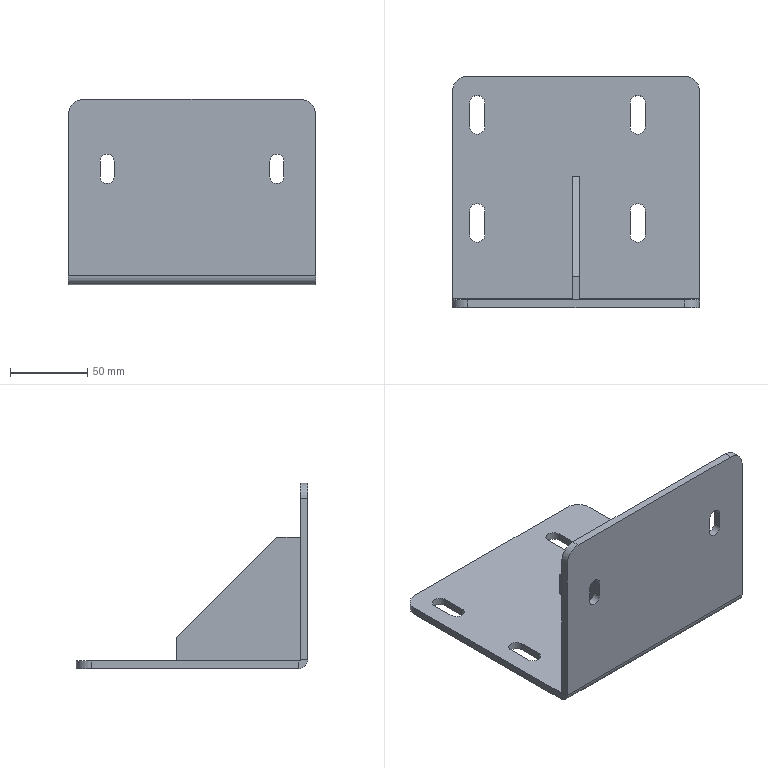Part | SolidWorks | features ICE 3, EdgeFlange 1, Fillet 1, FlatPattern 1, Gusset 1, SMBaseFlange 1, SheetMetal 1 | 2 solids | 51 faces | box 160 x 150 x 120 mm | volume 225790 mm3 | plane 31 | cylinder 20 | commonest cylinder face diameters 10 x8 9 x6 20 x4 1.473 x1 11.473 x1
STEP:
#1=CARTESIAN_POINT('',(-2.5,80.,-55.));
#2=VERTEX_POINT('',#1);
#3=CARTESIAN_POINT('',(-2.5,80.,-40.));
#4=VERTEX_POINT('',#3);
#5=CARTESIAN_POINT('',(-2.5,80.,-55.));
#6=DIRECTION('',(0.,0.,1.));
#7=VECTOR('',#6,1000.);
#8=LINE('',#5,#7);
#9=EDGE_CURVE('',#2,#4,#8,.T.);
#10=ORIENTED_EDGE('',*,*,#9,.T.);
#11=CARTESIAN_POINT('',(2.5,80.,-40.));
#12=VERTEX_POINT('',#11);
#13=CARTESIAN_POINT('',(2.5,80.,-40.));
#14=DIRECTION('',(-1.,0.,0.));
#15=VECTOR('',#14,1000.);
#16=LINE('',#13,#15);
#17=EDGE_CURVE('',#12,#4,#16,.T.);
#18=ORIENTED_EDGE('',*,*,#17,.F.);
#19=CARTESIAN_POINT('',(2.5,80.,-55.));
#20=VERTEX_POINT('',#19);
#21=CARTESIAN_POINT('',(2.5,80.,-55.));
#22=DIRECTION('',(0.,0.,1.));
#23=VECTOR('',#22,1000.);
#24=LINE('',#21,#23);
#25=EDGE_CURVE('',#20,#12,#24,.T.);
#26=ORIENTED_EDGE('',*,*,#25,.F.);
#27=CARTESIAN_POINT('',(2.5,80.,-55.));
#28=DIRECTION('',(-1.,0.,0.));
#29=VECTOR('',#28,1000.);
#30=LINE('',#27,#29);
#31=EDGE_CURVE('',#20,#2,#30,.T.);
#32=ORIENTED_EDGE('',*,*,#31,.T.);
#33=EDGE_LOOP('',(#10,#18,#26,#32));
#34=FACE_OUTER_BOUND('',#33,.T.);
#35=CARTESIAN_POINT('',(2.5,80.,-55.));
#36=DIRECTION('',(0.,-1.,0.));
#37=DIRECTION('',(0.,0.,-1.));
#38=AXIS2_PLACEMENT_3D('',#35,#36,#37);
#39=PLANE('',#38);
#40=ADVANCED_FACE('',(#34),#39,.F.);
#41=CARTESIAN_POINT('',(-2.5,15.,25.));
#42=VERTEX_POINT('',#41);
#43=CARTESIAN_POINT('',(-2.5,80.,-40.));
#44=DIRECTION('',(0.,-0.7071,0.7071));
#45=VECTOR('',#44,1000.);
#46=LINE('',#43,#45);
#47=EDGE_CURVE('',#4,#42,#46,.T.);
#48=ORIENTED_EDGE('',*,*,#47,.T.);
#49=CARTESIAN_POINT('',(2.5,15.,25.));
#50=VERTEX_POINT('',#49);
#51=CARTESIAN_POINT('',(2.5,15.,25.));
#52=DIRECTION('',(-1.,0.,0.));
#53=VECTOR('',#52,1000.);
#54=LINE('',#51,#53);
#55=EDGE_CURVE('',#50,#42,#54,.T.);
#56=ORIENTED_EDGE('',*,*,#55,.F.);
#57=CARTESIAN_POINT('',(2.5,80.,-40.));
#58=DIRECTION('',(0.,-0.7071,0.7071));
#59=VECTOR('',#58,1000.);
#60=LINE('',#57,#59);
#61=EDGE_CURVE('',#12,#50,#60,.T.);
#62=ORIENTED_EDGE('',*,*,#61,.F.);
#63=ORIENTED_EDGE('',*,*,#17,.T.);
#64=EDGE_LOOP('',(#48,#56,#62,#63));
#65=FACE_OUTER_BOUND('',#64,.T.);
#66=CARTESIAN_POINT('',(2.5,80.,-40.));
#67=DIRECTION('',(0.,-0.7071,-0.7071));
#68=DIRECTION('',(0.,0.7071,-0.7071));
#69=AXIS2_PLACEMENT_3D('',#66,#67,#68);
#70=PLANE('',#69);
#71=ADVANCED_FACE('',(#65),#70,.F.);
#72=CARTESIAN_POINT('',(-2.5,0.,25.));
#73=VERTEX_POINT('',#72);
#74=CARTESIAN_POINT('',(-2.5,0.,25.));
#75=DIRECTION('',(0.,-1.,0.));
#76=VECTOR('',#75,1000.);
#77=LINE('',#74,#76);
#78=EDGE_CURVE('',#42,#73,#77,.T.);
#79=ORIENTED_EDGE('',*,*,#78,.T.);
#80=CARTESIAN_POINT('',(2.5,0.,25.));
#81=VERTEX_POINT('',#80);
#82=CARTESIAN_POINT('',(2.5,0.,25.));
#83=DIRECTION('',(-1.,0.,0.));
#84=VECTOR('',#83,1000.);
#85=LINE('',#82,#84);
#86=EDGE_CURVE('',#81,#73,#85,.T.);
#87=ORIENTED_EDGE('',*,*,#86,.F.);
#88=CARTESIAN_POINT('',(2.5,0.,25.));
#89=DIRECTION('',(0.,-1.,0.));
#90=VECTOR('',#89,1000.);
#91=LINE('',#88,#90);
#92=EDGE_CURVE('',#50,#81,#91,.T.);
#93=ORIENTED_EDGE('',*,*,#92,.F.);
#94=ORIENTED_EDGE('',*,*,#55,.T.);
#95=EDGE_LOOP('',(#79,#87,#93,#94));
#96=FACE_OUTER_BOUND('',#95,.T.);
#97=CARTESIAN_POINT('',(2.5,0.,25.));
#98=DIRECTION('',(0.,0.,-1.));
#99=DIRECTION('',(-1.,0.,0.));
#100=AXIS2_PLACEMENT_3D('',#97,#98,#99);
#101=PLANE('',#100);
#102=ADVANCED_FACE('',(#96),#101,.F.);
#103=CARTESIAN_POINT('',(-2.5,0.,-55.));
#104=VERTEX_POINT('',#103);
#105=CARTESIAN_POINT('',(-2.5,0.,-55.));
#106=DIRECTION('',(0.,0.,-1.));
#107=VECTOR('',#106,1000.);
#108=LINE('',#105,#107);
#109=EDGE_CURVE('',#73,#104,#108,.T.);
#110=ORIENTED_EDGE('',*,*,#109,.T.);
#111=CARTESIAN_POINT('',(2.5,0.,-55.));
#112=VERTEX_POINT('',#111);
#113=CARTESIAN_POINT('',(2.5,0.,-55.));
#114=DIRECTION('',(-1.,0.,0.));
#115=VECTOR('',#114,1000.);
#116=LINE('',#113,#115);
#117=EDGE_CURVE('',#112,#104,#116,.T.);
#118=ORIENTED_EDGE('',*,*,#117,.F.);
#119=CARTESIAN_POINT('',(2.5,0.,-55.));
#120=DIRECTION('',(0.,0.,-1.));
#121=VECTOR('',#120,1000.);
#122=LINE('',#119,#121);
#123=EDGE_CURVE('',#81,#112,#122,.T.);
#124=ORIENTED_EDGE('',*,*,#123,.F.);
#125=ORIENTED_EDGE('',*,*,#86,.T.);
#126=EDGE_LOOP('',(#110,#118,#124,#125));
#127=FACE_OUTER_BOUND('',#126,.T.);
#128=CARTESIAN_POINT('',(2.5,0.,-55.));
#129=DIRECTION('',(0.,1.,0.));
#130=DIRECTION('',(0.,0.,1.));
#131=AXIS2_PLACEMENT_3D('',#128,#129,#130);
#132=PLANE('',#131);
#133=ADVANCED_FACE('',(#127),#132,.F.);
#134=CARTESIAN_POINT('',(-2.5,0.,-55.));
#135=DIRECTION('',(0.,1.,0.));
#136=VECTOR('',#135,1000.);
#137=LINE('',#134,#136);
#138=EDGE_CURVE('',#104,#2,#137,.T.);
#139=ORIENTED_EDGE('',*,*,#138,.T.);
#140=ORIENTED_EDGE('',*,*,#31,.F.);
#141=CARTESIAN_POINT('',(2.5,0.,-55.));
#142=DIRECTION('',(0.,1.,0.));
#143=VECTOR('',#142,1000.);
#144=LINE('',#141,#143);
#145=EDGE_CURVE('',#112,#20,#144,.T.);
#146=ORIENTED_EDGE('',*,*,#145,.F.);
#147=ORIENTED_EDGE('',*,*,#117,.T.);
#148=EDGE_LOOP('',(#139,#140,#146,#147));
#149=FACE_OUTER_BOUND('',#148,.T.);
#150=CARTESIAN_POINT('',(2.5,0.,-55.));
#151=DIRECTION('',(0.,0.,1.));
#152=DIRECTION('',(1.,0.,0.));
#153=AXIS2_PLACEMENT_3D('',#150,#151,#152);
#154=PLANE('',#153);
#155=ADVANCED_FACE('',(#149),#154,.F.);
#156=ORIENTED_EDGE('',*,*,#25,.T.);
#157=ORIENTED_EDGE('',*,*,#61,.T.);
#158=ORIENTED_EDGE('',*,*,#92,.T.);
#159=ORIENTED_EDGE('',*,*,#123,.T.);
#160=ORIENTED_EDGE('',*,*,#145,.T.);
#161=EDGE_LOOP('',(#156,#157,#158,#159,#160));
#162=FACE_OUTER_BOUND('',#161,.T.);
#163=CARTESIAN_POINT('',(2.5,0.,0.));
#164=DIRECTION('',(-1.,0.,0.));
#165=DIRECTION('',(0.,0.,1.));
#166=AXIS2_PLACEMENT_3D('',#163,#164,#165);
#167=PLANE('',#166);
#168=ADVANCED_FACE('',(#162),#167,.F.);
#169=ORIENTED_EDGE('',*,*,#9,.F.);
#170=ORIENTED_EDGE('',*,*,#138,.F.);
#171=ORIENTED_EDGE('',*,*,#109,.F.);
#172=ORIENTED_EDGE('',*,*,#78,.F.);
#173=ORIENTED_EDGE('',*,*,#47,.F.);
#174=EDGE_LOOP('',(#169,#170,#171,#172,#173));
#175=FACE_OUTER_BOUND('',#174,.T.);
#176=CARTESIAN_POINT('',(-2.5,0.,0.));
#177=DIRECTION('',(-1.,0.,0.));
#178=DIRECTION('',(0.,0.,1.));
#179=AXIS2_PLACEMENT_3D('',#176,#177,#178);
#180=PLANE('',#179);
#181=ADVANCED_FACE('',(#175),#180,.T.);
#182=CLOSED_SHELL('',(#40,#71,#102,#133,#155,#168,#181));
#183=MANIFOLD_SOLID_BREP('',#182);
#184=CARTESIAN_POINT('',(-55.,-5.,24.5));
#185=VERTEX_POINT('',#184);
#186=CARTESIAN_POINT('',(-50.5,-5.,20.));
#187=VERTEX_POINT('',#186);
#188=CARTESIAN_POINT('',(-55.,-5.,20.));
#189=DIRECTION('',(0.,1.,0.));
#190=DIRECTION('',(0.,0.,1.));
#191=AXIS2_PLACEMENT_3D('',#188,#189,#190);
#192=CIRCLE('',#191,4.5);
#193=EDGE_CURVE('',#185,#187,#192,.T.);
#194=ORIENTED_EDGE('',*,*,#193,.F.);
#195=CARTESIAN_POINT('',(-55.,0.,24.5));
#196=VERTEX_POINT('',#195);
#197=CARTESIAN_POINT('',(-55.,-5.,24.5));
#198=DIRECTION('',(0.,1.,0.));
#199=VECTOR('',#198,1000.);
#200=LINE('',#197,#199);
#201=EDGE_CURVE('',#185,#196,#200,.T.);
#202=ORIENTED_EDGE('',*,*,#201,.T.);
#203=CARTESIAN_POINT('',(-50.5,0.,20.));
#204=VERTEX_POINT('',#203);
#205=CARTESIAN_POINT('',(-55.,0.,20.));
#206=DIRECTION('',(0.,1.,0.));
#207=DIRECTION('',(0.,0.,1.));
#208=AXIS2_PLACEMENT_3D('',#205,#206,#207);
#209=CIRCLE('',#208,4.5);
#210=EDGE_CURVE('',#196,#204,#209,.T.);
#211=ORIENTED_EDGE('',*,*,#210,.T.);
#212=CARTESIAN_POINT('',(-50.5,-5.,20.));
#213=DIRECTION('',(0.,1.,0.));
#214=VECTOR('',#213,1000.);
#215=LINE('',#212,#214);
#216=EDGE_CURVE('',#187,#204,#215,.T.);
#217=ORIENTED_EDGE('',*,*,#216,.F.);
#218=EDGE_LOOP('',(#194,#202,#211,#217));
#219=FACE_OUTER_BOUND('',#218,.T.);
#220=CARTESIAN_POINT('',(-55.,-5.,20.));
#221=DIRECTION('',(0.,1.,0.));
#222=DIRECTION('',(0.,0.,1.));
#223=AXIS2_PLACEMENT_3D('',#220,#221,#222);
#224=CYLINDRICAL_SURFACE('',#223,4.5);
#225=ADVANCED_FACE('',(#219),#224,.F.);
#226=CARTESIAN_POINT('',(55.,-5.,24.5));
#227=VERTEX_POINT('',#226);
#228=CARTESIAN_POINT('',(59.5,-5.,20.));
#229=VERTEX_POINT('',#228);
#230=CARTESIAN_POINT('',(55.,-5.,20.));
#231=DIRECTION('',(0.,1.,0.));
#232=DIRECTION('',(0.,0.,1.));
#233=AXIS2_PLACEMENT_3D('',#230,#231,#232);
#234=CIRCLE('',#233,4.5);
#235=EDGE_CURVE('',#227,#229,#234,.T.);
#236=ORIENTED_EDGE('',*,*,#235,.F.);
#237=CARTESIAN_POINT('',(55.,0.,24.5));
#238=VERTEX_POINT('',#237);
#239=CARTESIAN_POINT('',(55.,-5.,24.5));
#240=DIRECTION('',(0.,1.,0.));
#241=VECTOR('',#240,1000.);
#242=LINE('',#239,#241);
#243=EDGE_CURVE('',#227,#238,#242,.T.);
#244=ORIENTED_EDGE('',*,*,#243,.T.);
#245=CARTESIAN_POINT('',(59.5,0.,20.));
#246=VERTEX_POINT('',#245);
#247=CARTESIAN_POINT('',(55.,0.,20.));
#248=DIRECTION('',(0.,1.,0.));
#249=DIRECTION('',(0.,0.,1.));
#250=AXIS2_PLACEMENT_3D('',#247,#248,#249);
#251=CIRCLE('',#250,4.5);
#252=EDGE_CURVE('',#238,#246,#251,.T.);
#253=ORIENTED_EDGE('',*,*,#252,.T.);
#254=CARTESIAN_POINT('',(59.5,-5.,20.));
#255=DIRECTION('',(0.,1.,0.));
#256=VECTOR('',#255,1000.);
#257=LINE('',#254,#256);
#258=EDGE_CURVE('',#229,#246,#257,.T.);
#259=ORIENTED_EDGE('',*,*,#258,.F.);
#260=EDGE_LOOP('',(#236,#244,#253,#259));
#261=FACE_OUTER_BOUND('',#260,.T.);
#262=CARTESIAN_POINT('',(55.,-5.,20.));
#263=DIRECTION('',(0.,1.,0.));
#264=DIRECTION('',(0.,0.,1.));
#265=AXIS2_PLACEMENT_3D('',#262,#263,#264);
#266=CYLINDRICAL_SURFACE('',#265,4.5);
#267=ADVANCED_FACE('',(#261),#266,.F.);
#268=CARTESIAN_POINT('',(-80.,0.,-54.263));
#269=VERTEX_POINT('',#268);
#270=CARTESIAN_POINT('',(-80.,0.,50.));
#271=VERTEX_POINT('',#270);
#272=CARTESIAN_POINT('',(-80.,0.,50.));
#273=DIRECTION('',(0.,0.,1.));
#274=VECTOR('',#273,1000.);
#275=LINE('',#272,#274);
#276=EDGE_CURVE('',#269,#271,#275,.T.);
#277=ORIENTED_EDGE('',*,*,#276,.F.);
#278=CARTESIAN_POINT('',(-80.,-5.,-54.263));
#279=VERTEX_POINT('',#278);
#280=CARTESIAN_POINT('',(-80.,0.,-54.263));
#281=DIRECTION('',(0.,-1.,0.));
#282=VECTOR('',#281,1000.);
#283=LINE('',#280,#282);
#284=EDGE_CURVE('',#269,#279,#283,.T.);
#285=ORIENTED_EDGE('',*,*,#284,.T.);
#286=CARTESIAN_POINT('',(-80.,-5.,50.));
#287=VERTEX_POINT('',#286);
#288=CARTESIAN_POINT('',(-80.,-5.,50.));
#289=DIRECTION('',(0.,0.,1.));
#290=VECTOR('',#289,1000.);
#291=LINE('',#288,#290);
#292=EDGE_CURVE('',#279,#287,#291,.T.);
#293=ORIENTED_EDGE('',*,*,#292,.T.);
#294=CARTESIAN_POINT('',(-80.,-5.,50.));
#295=DIRECTION('',(0.,1.,0.));
#296=VECTOR('',#295,1000.);
#297=LINE('',#294,#296);
#298=EDGE_CURVE('',#287,#271,#297,.T.);
#299=ORIENTED_EDGE('',*,*,#298,.T.);
#300=EDGE_LOOP('',(#277,#285,#293,#299));
#301=FACE_OUTER_BOUND('',#300,.T.);
#302=CARTESIAN_POINT('',(-80.,-5.,50.));
#303=DIRECTION('',(-1.,0.,0.));
#304=DIRECTION('',(0.,0.,1.));
#305=AXIS2_PLACEMENT_3D('',#302,#303,#304);
#306=PLANE('',#305);
#307=ADVANCED_FACE('',(#301),#306,.T.);
#308=CARTESIAN_POINT('',(-50.5,-5.,10.));
#309=VERTEX_POINT('',#308);
#310=CARTESIAN_POINT('',(-59.5,-5.,10.));
#311=VERTEX_POINT('',#310);
#312=CARTESIAN_POINT('',(-55.,-5.,10.));
#313=DIRECTION('',(0.,1.,0.));
#314=DIRECTION('',(0.,0.,1.));
#315=AXIS2_PLACEMENT_3D('',#312,#313,#314);
#316=CIRCLE('',#315,4.5);
#317=EDGE_CURVE('',#309,#311,#316,.T.);
#318=ORIENTED_EDGE('',*,*,#317,.T.);
#319=CARTESIAN_POINT('',(-59.5,-5.,20.));
#320=VERTEX_POINT('',#319);
#321=CARTESIAN_POINT('',(-59.5,-5.,10.));
#322=DIRECTION('',(0.,0.,1.));
#323=VECTOR('',#322,1000.);
#324=LINE('',#321,#323);
#325=EDGE_CURVE('',#311,#320,#324,.T.);
#326=ORIENTED_EDGE('',*,*,#325,.T.);
#327=CARTESIAN_POINT('',(-55.,-5.,20.));
#328=DIRECTION('',(0.,1.,0.));
#329=DIRECTION('',(0.,0.,1.));
#330=AXIS2_PLACEMENT_3D('',#327,#328,#329);
#331=CIRCLE('',#330,4.5);
#332=EDGE_CURVE('',#320,#185,#331,.T.);
#333=ORIENTED_EDGE('',*,*,#332,.T.);
#334=ORIENTED_EDGE('',*,*,#193,.T.);
#335=CARTESIAN_POINT('',(-50.5,-5.,10.));
#336=DIRECTION('',(0.,0.,-1.));
#337=VECTOR('',#336,1000.);
#338=LINE('',#335,#337);
#339=EDGE_CURVE('',#187,#309,#338,.T.);
#340=ORIENTED_EDGE('',*,*,#339,.T.);
#341=EDGE_LOOP('',(#318,#326,#333,#334,#340));
#342=FACE_BOUND('',#341,.T.);
#343=CARTESIAN_POINT('',(59.5,-5.,10.));
#344=VERTEX_POINT('',#343);
#345=CARTESIAN_POINT('',(50.5,-5.,10.));
#346=VERTEX_POINT('',#345);
#347=CARTESIAN_POINT('',(55.,-5.,10.));
#348=DIRECTION('',(0.,1.,0.));
#349=DIRECTION('',(0.,0.,1.));
#350=AXIS2_PLACEMENT_3D('',#347,#348,#349);
#351=CIRCLE('',#350,4.5);
#352=EDGE_CURVE('',#344,#346,#351,.T.);
#353=ORIENTED_EDGE('',*,*,#352,.T.);
#354=CARTESIAN_POINT('',(50.5,-5.,20.));
#355=VERTEX_POINT('',#354);
#356=CARTESIAN_POINT('',(50.5,-5.,10.));
#357=DIRECTION('',(0.,0.,1.));
#358=VECTOR('',#357,1000.);
#359=LINE('',#356,#358);
#360=EDGE_CURVE('',#346,#355,#359,.T.);
#361=ORIENTED_EDGE('',*,*,#360,.T.);
#362=CARTESIAN_POINT('',(55.,-5.,20.));
#363=DIRECTION('',(0.,1.,0.));
#364=DIRECTION('',(0.,0.,1.));
#365=AXIS2_PLACEMENT_3D('',#362,#363,#364);
#366=CIRCLE('',#365,4.5);
#367=EDGE_CURVE('',#355,#227,#366,.T.);
#368=ORIENTED_EDGE('',*,*,#367,.T.);
#369=ORIENTED_EDGE('',*,*,#235,.T.);
#370=CARTESIAN_POINT('',(59.5,-5.,10.));
#371=DIRECTION('',(0.,0.,-1.));
#372=VECTOR('',#371,1000.);
#373=LINE('',#370,#372);
#374=EDGE_CURVE('',#229,#344,#373,.T.);
#375=ORIENTED_EDGE('',*,*,#374,.T.);
#376=EDGE_LOOP('',(#353,#361,#368,#369,#375));
#377=FACE_BOUND('',#376,.T.);
#378=ORIENTED_EDGE('',*,*,#292,.F.);
#379=CARTESIAN_POINT('',(80.,-5.,-54.263));
#380=VERTEX_POINT('',#379);
#381=CARTESIAN_POINT('',(-80.,-5.,-54.263));
#382=DIRECTION('',(1.,0.,0.));
#383=VECTOR('',#382,1000.);
#384=LINE('',#381,#383);
#385=EDGE_CURVE('',#279,#380,#384,.T.);
#386=ORIENTED_EDGE('',*,*,#385,.T.);
#387=CARTESIAN_POINT('',(80.,-5.,50.));
#388=VERTEX_POINT('',#387);
#389=CARTESIAN_POINT('',(80.,-5.,50.));
#390=DIRECTION('',(0.,0.,-1.));
#391=VECTOR('',#390,1000.);
#392=LINE('',#389,#391);
#393=EDGE_CURVE('',#388,#380,#392,.T.);
#394=ORIENTED_EDGE('',*,*,#393,.F.);
#395=CARTESIAN_POINT('',(70.,-5.,60.));
#396=VERTEX_POINT('',#395);
#397=CARTESIAN_POINT('',(70.,-5.,50.));
#398=DIRECTION('',(0.,1.,0.));
#399=DIRECTION('',(0.,0.,-1.));
#400=AXIS2_PLACEMENT_3D('',#397,#398,#399);
#401=CIRCLE('',#400,10.);
#402=EDGE_CURVE('',#396,#388,#401,.T.);
#403=ORIENTED_EDGE('',*,*,#402,.F.);
#404=CARTESIAN_POINT('',(-70.,-5.,60.));
#405=VERTEX_POINT('',#404);
#406=CARTESIAN_POINT('',(-70.,-5.,60.));
#407=DIRECTION('',(1.,0.,0.));
#408=VECTOR('',#407,1000.);
#409=LINE('',#406,#408);
#410=EDGE_CURVE('',#405,#396,#409,.T.);
#411=ORIENTED_EDGE('',*,*,#410,.F.);
#412=CARTESIAN_POINT('',(-70.,-5.,50.));
#413=DIRECTION('',(0.,1.,0.));
#414=DIRECTION('',(0.,0.,-1.));
#415=AXIS2_PLACEMENT_3D('',#412,#413,#414);
#416=CIRCLE('',#415,10.);
#417=EDGE_CURVE('',#287,#405,#416,.T.);
#418=ORIENTED_EDGE('',*,*,#417,.F.);
#419=EDGE_LOOP('',(#378,#386,#394,#403,#411,#418));
#420=FACE_OUTER_BOUND('',#419,.T.);
#421=CARTESIAN_POINT('',(-70.,-5.,50.));
#422=DIRECTION('',(0.,-1.,0.));
#423=DIRECTION('',(0.,0.,-1.));
#424=AXIS2_PLACEMENT_3D('',#421,#422,#423);
#425=PLANE('',#424);
#426=ADVANCED_FACE('',(#342,#377,#420),#425,.T.);
#427=CARTESIAN_POINT('',(-59.5,0.,10.));
#428=VERTEX_POINT('',#427);
#429=CARTESIAN_POINT('',(-59.5,0.,20.));
#430=VERTEX_POINT('',#429);
#431=CARTESIAN_POINT('',(-59.5,0.,10.));
#432=DIRECTION('',(0.,0.,1.));
#433=VECTOR('',#432,1000.);
#434=LINE('',#431,#433);
#435=EDGE_CURVE('',#428,#430,#434,.T.);
#436=ORIENTED_EDGE('',*,*,#435,.F.);
#437=CARTESIAN_POINT('',(-50.5,0.,10.));
#438=VERTEX_POINT('',#437);
#439=CARTESIAN_POINT('',(-55.,0.,10.));
#440=DIRECTION('',(0.,1.,0.));
#441=DIRECTION('',(0.,0.,1.));
#442=AXIS2_PLACEMENT_3D('',#439,#440,#441);
#443=CIRCLE('',#442,4.5);
#444=EDGE_CURVE('',#438,#428,#443,.T.);
#445=ORIENTED_EDGE('',*,*,#444,.F.);
#446=CARTESIAN_POINT('',(-50.5,0.,10.));
#447=DIRECTION('',(0.,0.,-1.));
#448=VECTOR('',#447,1000.);
#449=LINE('',#446,#448);
#450=EDGE_CURVE('',#204,#438,#449,.T.);
#451=ORIENTED_EDGE('',*,*,#450,.F.);
#452=ORIENTED_EDGE('',*,*,#210,.F.);
#453=CARTESIAN_POINT('',(-55.,0.,20.));
#454=DIRECTION('',(0.,1.,0.));
#455=DIRECTION('',(0.,0.,1.));
#456=AXIS2_PLACEMENT_3D('',#453,#454,#455);
#457=CIRCLE('',#456,4.5);
#458=EDGE_CURVE('',#430,#196,#457,.T.);
#459=ORIENTED_EDGE('',*,*,#458,.F.);
#460=EDGE_LOOP('',(#436,#445,#451,#452,#459));
#461=FACE_BOUND('',#460,.T.);
#462=CARTESIAN_POINT('',(50.5,0.,10.));
#463=VERTEX_POINT('',#462);
#464=CARTESIAN_POINT('',(50.5,0.,20.));
#465=VERTEX_POINT('',#464);
#466=CARTESIAN_POINT('',(50.5,0.,10.));
#467=DIRECTION('',(0.,0.,1.));
#468=VECTOR('',#467,1000.);
#469=LINE('',#466,#468);
#470=EDGE_CURVE('',#463,#465,#469,.T.);
#471=ORIENTED_EDGE('',*,*,#470,.F.);
#472=CARTESIAN_POINT('',(59.5,0.,10.));
#473=VERTEX_POINT('',#472);
#474=CARTESIAN_POINT('',(55.,0.,10.));
#475=DIRECTION('',(0.,1.,0.));
#476=DIRECTION('',(0.,0.,1.));
#477=AXIS2_PLACEMENT_3D('',#474,#475,#476);
#478=CIRCLE('',#477,4.5);
#479=EDGE_CURVE('',#473,#463,#478,.T.);
#480=ORIENTED_EDGE('',*,*,#479,.F.);
#481=CARTESIAN_POINT('',(59.5,0.,10.));
#482=DIRECTION('',(0.,0.,-1.));
#483=VECTOR('',#482,1000.);
#484=LINE('',#481,#483);
#485=EDGE_CURVE('',#246,#473,#484,.T.);
#486=ORIENTED_EDGE('',*,*,#485,.F.);
#487=ORIENTED_EDGE('',*,*,#252,.F.);
#488=CARTESIAN_POINT('',(55.,0.,20.));
#489=DIRECTION('',(0.,1.,0.));
#490=DIRECTION('',(0.,0.,1.));
#491=AXIS2_PLACEMENT_3D('',#488,#489,#490);
#492=CIRCLE('',#491,4.5);
#493=EDGE_CURVE('',#465,#238,#492,.T.);
#494=ORIENTED_EDGE('',*,*,#493,.F.);
#495=EDGE_LOOP('',(#471,#480,#486,#487,#494));
#496=FACE_BOUND('',#495,.T.);
#497=CARTESIAN_POINT('',(80.,0.,-54.263));
#498=VERTEX_POINT('',#497);
#499=CARTESIAN_POINT('',(-80.,0.,-54.263));
#500=DIRECTION('',(1.,0.,0.));
#501=VECTOR('',#500,1000.);
#502=LINE('',#499,#501);
#503=EDGE_CURVE('',#269,#498,#502,.T.);
#504=ORIENTED_EDGE('',*,*,#503,.F.);
#505=ORIENTED_EDGE('',*,*,#276,.T.);
#506=CARTESIAN_POINT('',(-70.,0.,60.));
#507=VERTEX_POINT('',#506);
#508=CARTESIAN_POINT('',(-70.,0.,50.));
#509=DIRECTION('',(0.,1.,0.));
#510=DIRECTION('',(0.,0.,-1.));
#511=AXIS2_PLACEMENT_3D('',#508,#509,#510);
#512=CIRCLE('',#511,10.);
#513=EDGE_CURVE('',#271,#507,#512,.T.);
#514=ORIENTED_EDGE('',*,*,#513,.T.);
#515=CARTESIAN_POINT('',(70.,0.,60.));
#516=VERTEX_POINT('',#515);
#517=CARTESIAN_POINT('',(-70.,0.,60.));
#518=DIRECTION('',(1.,0.,0.));
#519=VECTOR('',#518,1000.);
#520=LINE('',#517,#519);
#521=EDGE_CURVE('',#507,#516,#520,.T.);
#522=ORIENTED_EDGE('',*,*,#521,.T.);
#523=CARTESIAN_POINT('',(80.,0.,50.));
#524=VERTEX_POINT('',#523);
#525=CARTESIAN_POINT('',(70.,0.,50.));
#526=DIRECTION('',(0.,1.,0.));
#527=DIRECTION('',(0.,0.,-1.));
#528=AXIS2_PLACEMENT_3D('',#525,#526,#527);
#529=CIRCLE('',#528,10.);
#530=EDGE_CURVE('',#516,#524,#529,.T.);
#531=ORIENTED_EDGE('',*,*,#530,.T.);
#532=CARTESIAN_POINT('',(80.,0.,50.));
#533=DIRECTION('',(0.,0.,-1.));
#534=VECTOR('',#533,1000.);
#535=LINE('',#532,#534);
#536=EDGE_CURVE('',#524,#498,#535,.T.);
#537=ORIENTED_EDGE('',*,*,#536,.T.);
#538=EDGE_LOOP('',(#504,#505,#514,#522,#531,#537));
#539=FACE_OUTER_BOUND('',#538,.T.);
#540=CARTESIAN_POINT('',(-70.,0.,50.));
#541=DIRECTION('',(0.,-1.,0.));
#542=DIRECTION('',(0.,0.,-1.));
#543=AXIS2_PLACEMENT_3D('',#540,#541,#542);
#544=PLANE('',#543);
#545=ADVANCED_FACE('',(#461,#496,#539),#544,.F.);
#546=CARTESIAN_POINT('',(80.,0.,-54.263));
#547=DIRECTION('',(0.,-1.,0.));
#548=VECTOR('',#547,1000.);
#549=LINE('',#546,#548);
#550=EDGE_CURVE('',#498,#380,#549,.T.);
#551=ORIENTED_EDGE('',*,*,#550,.F.);
#552=ORIENTED_EDGE('',*,*,#536,.F.);
#553=CARTESIAN_POINT('',(80.,-5.,50.));
#554=DIRECTION('',(0.,1.,0.));
#555=VECTOR('',#554,1000.);
#556=LINE('',#553,#555);
#557=EDGE_CURVE('',#388,#524,#556,.T.);
#558=ORIENTED_EDGE('',*,*,#557,.F.);
#559=ORIENTED_EDGE('',*,*,#393,.T.);
#560=EDGE_LOOP('',(#551,#552,#558,#559));
#561=FACE_OUTER_BOUND('',#560,.T.);
#562=CARTESIAN_POINT('',(80.,-5.,50.));
#563=DIRECTION('',(1.,0.,0.));
#564=DIRECTION('',(0.,0.,-1.));
#565=AXIS2_PLACEMENT_3D('',#562,#563,#564);
#566=PLANE('',#565);
#567=ADVANCED_FACE('',(#561),#566,.T.);
#568=ORIENTED_EDGE('',*,*,#530,.F.);
#569=CARTESIAN_POINT('',(70.,-5.,60.));
#570=DIRECTION('',(0.,1.,0.));
#571=VECTOR('',#570,1000.);
#572=LINE('',#569,#571);
#573=EDGE_CURVE('',#396,#516,#572,.T.);
#574=ORIENTED_EDGE('',*,*,#573,.F.);
#575=ORIENTED_EDGE('',*,*,#402,.T.);
#576=ORIENTED_EDGE('',*,*,#557,.T.);
#577=EDGE_LOOP('',(#568,#574,#575,#576));
#578=FACE_OUTER_BOUND('',#577,.T.);
#579=CARTESIAN_POINT('',(70.,-5.,50.));
#580=DIRECTION('',(0.,1.,0.));
#581=DIRECTION('',(0.,0.,1.));
#582=AXIS2_PLACEMENT_3D('',#579,#580,#581);
#583=CYLINDRICAL_SURFACE('',#582,10.);
#584=ADVANCED_FACE('',(#578),#583,.T.);
#585=ORIENTED_EDGE('',*,*,#521,.F.);
#586=CARTESIAN_POINT('',(-70.,-5.,60.));
#587=DIRECTION('',(0.,1.,0.));
#588=VECTOR('',#587,1000.);
#589=LINE('',#586,#588);
#590=EDGE_CURVE('',#405,#507,#589,.T.);
#591=ORIENTED_EDGE('',*,*,#590,.F.);
#592=ORIENTED_EDGE('',*,*,#410,.T.);
#593=ORIENTED_EDGE('',*,*,#573,.T.);
#594=EDGE_LOOP('',(#585,#591,#592,#593));
#595=FACE_OUTER_BOUND('',#594,.T.);
#596=CARTESIAN_POINT('',(-70.,-5.,60.));
#597=DIRECTION('',(0.,0.,1.));
#598=DIRECTION('',(1.,0.,0.));
#599=AXIS2_PLACEMENT_3D('',#596,#597,#598);
#600=PLANE('',#599);
#601=ADVANCED_FACE('',(#595),#600,.T.);
#602=ORIENTED_EDGE('',*,*,#513,.F.);
#603=ORIENTED_EDGE('',*,*,#298,.F.);
#604=ORIENTED_EDGE('',*,*,#417,.T.);
#605=ORIENTED_EDGE('',*,*,#590,.T.);
#606=EDGE_LOOP('',(#602,#603,#604,#605));
#607=FACE_OUTER_BOUND('',#606,.T.);
#608=CARTESIAN_POINT('',(-70.,-5.,50.));
#609=DIRECTION('',(0.,1.,0.));
#610=DIRECTION('',(0.,0.,1.));
#611=AXIS2_PLACEMENT_3D('',#608,#609,#610);
#612=CYLINDRICAL_SURFACE('',#611,10.);
#613=ADVANCED_FACE('',(#607),#612,.T.);
#614=CARTESIAN_POINT('',(80.,0.7366,-55.));
#615=VERTEX_POINT('',#614);
#616=CARTESIAN_POINT('',(80.,0.7366,-60.));
#617=VERTEX_POINT('',#616);
#618=CARTESIAN_POINT('',(80.,0.7366,-60.));
#619=DIRECTION('',(0.,0.,-1.));
#620=VECTOR('',#619,1000.);
#621=LINE('',#618,#620);
#622=EDGE_CURVE('',#615,#617,#621,.T.);
#623=ORIENTED_EDGE('',*,*,#622,.F.);
#624=CARTESIAN_POINT('',(80.,0.7366,-54.263));
#625=DIRECTION('',(1.,0.,0.));
#626=DIRECTION('',(0.,-1.,0.));
#627=AXIS2_PLACEMENT_3D('',#624,#625,#626);
#628=CIRCLE('',#627,0.7366);
#629=EDGE_CURVE('',#498,#615,#628,.T.);
#630=ORIENTED_EDGE('',*,*,#629,.F.);
#631=ORIENTED_EDGE('',*,*,#550,.T.);
#632=CARTESIAN_POINT('',(80.,0.7366,-54.263));
#633=DIRECTION('',(1.,0.,0.));
#634=DIRECTION('',(0.,-1.,0.));
#635=AXIS2_PLACEMENT_3D('',#632,#633,#634);
#636=CIRCLE('',#635,5.737);
#637=EDGE_CURVE('',#380,#617,#636,.T.);
#638=ORIENTED_EDGE('',*,*,#637,.T.);
#639=EDGE_LOOP('',(#623,#630,#631,#638));
#640=FACE_OUTER_BOUND('',#639,.T.);
#641=CARTESIAN_POINT('',(80.,0.7366,-54.263));
#642=DIRECTION('',(1.,0.,0.));
#643=DIRECTION('',(0.,1.,0.));
#644=AXIS2_PLACEMENT_3D('',#641,#642,#643);
#645=PLANE('',#644);
#646=ADVANCED_FACE('',(#640),#645,.T.);
#647=CARTESIAN_POINT('',(-80.,0.7366,-55.));
#648=VERTEX_POINT('',#647);
#649=CARTESIAN_POINT('',(-80.,0.7366,-54.263));
#650=DIRECTION('',(-1.,0.,0.));
#651=DIRECTION('',(0.,-1.,0.));
#652=AXIS2_PLACEMENT_3D('',#649,#650,#651);
#653=CIRCLE('',#652,0.7366);
#654=EDGE_CURVE('',#648,#269,#653,.T.);
#655=ORIENTED_EDGE('',*,*,#654,.F.);
#656=CARTESIAN_POINT('',(-80.,0.7366,-60.));
#657=VERTEX_POINT('',#656);
#658=CARTESIAN_POINT('',(-80.,0.7366,-55.));
#659=DIRECTION('',(0.,0.,-1.));
#660=VECTOR('',#659,1000.);
#661=LINE('',#658,#660);
#662=EDGE_CURVE('',#648,#657,#661,.T.);
#663=ORIENTED_EDGE('',*,*,#662,.T.);
#664=CARTESIAN_POINT('',(-80.,0.7366,-54.263));
#665=DIRECTION('',(-1.,0.,0.));
#666=DIRECTION('',(0.,-1.,0.));
#667=AXIS2_PLACEMENT_3D('',#664,#665,#666);
#668=CIRCLE('',#667,5.737);
#669=EDGE_CURVE('',#657,#279,#668,.T.);
#670=ORIENTED_EDGE('',*,*,#669,.T.);
#671=ORIENTED_EDGE('',*,*,#284,.F.);
#672=EDGE_LOOP('',(#655,#663,#670,#671));
#673=FACE_OUTER_BOUND('',#672,.T.);
#674=CARTESIAN_POINT('',(-80.,0.7366,-54.263));
#675=DIRECTION('',(1.,0.,0.));
#676=DIRECTION('',(0.,1.,0.));
#677=AXIS2_PLACEMENT_3D('',#674,#675,#676);
#678=PLANE('',#677);
#679=ADVANCED_FACE('',(#673),#678,.F.);
#680=ORIENTED_EDGE('',*,*,#385,.F.);
#681=ORIENTED_EDGE('',*,*,#669,.F.);
#682=CARTESIAN_POINT('',(0.,0.7366,-60.));
#683=DIRECTION('',(-1.,0.,0.));
#684=VECTOR('',#683,1000.);
#685=LINE('',#682,#684);
#686=EDGE_CURVE('',#617,#657,#685,.T.);
#687=ORIENTED_EDGE('',*,*,#686,.F.);
#688=ORIENTED_EDGE('',*,*,#637,.F.);
#689=EDGE_LOOP('',(#680,#681,#687,#688));
#690=FACE_OUTER_BOUND('',#689,.T.);
#691=CARTESIAN_POINT('',(-80.,0.7366,-54.263));
#692=DIRECTION('',(-1.,0.,0.));
#693=DIRECTION('',(0.,0.,-1.));
#694=AXIS2_PLACEMENT_3D('',#691,#692,#693);
#695=CYLINDRICAL_SURFACE('',#694,5.737);
#696=ADVANCED_FACE('',(#690),#695,.T.);
#697=ORIENTED_EDGE('',*,*,#503,.T.);
#698=ORIENTED_EDGE('',*,*,#629,.T.);
#699=CARTESIAN_POINT('',(80.,0.7366,-55.));
#700=DIRECTION('',(-1.,0.,0.));
#701=VECTOR('',#700,1000.);
#702=LINE('',#699,#701);
#703=EDGE_CURVE('',#615,#648,#702,.T.);
#704=ORIENTED_EDGE('',*,*,#703,.T.);
#705=ORIENTED_EDGE('',*,*,#654,.T.);
#706=EDGE_LOOP('',(#697,#698,#704,#705));
#707=FACE_OUTER_BOUND('',#706,.T.);
#708=CARTESIAN_POINT('',(-80.,0.7366,-54.263));
#709=DIRECTION('',(-1.,0.,0.));
#710=DIRECTION('',(0.,0.,-1.));
#711=AXIS2_PLACEMENT_3D('',#708,#709,#710);
#712=CYLINDRICAL_SURFACE('',#711,0.7366);
#713=ADVANCED_FACE('',(#707),#712,.F.);
#714=CARTESIAN_POINT('',(-80.,135.,-55.));
#715=VERTEX_POINT('',#714);
#716=CARTESIAN_POINT('',(-80.,0.,-55.));
#717=DIRECTION('',(0.,-1.,0.));
#718=VECTOR('',#717,1000.);
#719=LINE('',#716,#718);
#720=EDGE_CURVE('',#715,#648,#719,.T.);
#721=ORIENTED_EDGE('',*,*,#720,.F.);
#722=CARTESIAN_POINT('',(-80.,135.,-60.));
#723=VERTEX_POINT('',#722);
#724=CARTESIAN_POINT('',(-80.,135.,-60.));
#725=DIRECTION('',(0.,0.,-1.));
#726=VECTOR('',#725,1000.);
#727=LINE('',#724,#726);
#728=EDGE_CURVE('',#715,#723,#727,.T.);
#729=ORIENTED_EDGE('',*,*,#728,.T.);
#730=CARTESIAN_POINT('',(-80.,0.,-60.));
#731=DIRECTION('',(0.,-1.,0.));
#732=VECTOR('',#731,1000.);
#733=LINE('',#730,#732);
#734=EDGE_CURVE('',#723,#657,#733,.T.);
#735=ORIENTED_EDGE('',*,*,#734,.T.);
#736=ORIENTED_EDGE('',*,*,#662,.F.);
#737=EDGE_LOOP('',(#721,#729,#735,#736));
#738=FACE_OUTER_BOUND('',#737,.T.);
#739=CARTESIAN_POINT('',(-80.,0.,-60.));
#740=DIRECTION('',(-1.,0.,0.));
#741=DIRECTION('',(0.,0.,1.));
#742=AXIS2_PLACEMENT_3D('',#739,#740,#741);
#743=PLANE('',#742);
#744=ADVANCED_FACE('',(#738),#743,.T.);
#745=CARTESIAN_POINT('',(80.,135.,-60.));
#746=VERTEX_POINT('',#745);
#747=CARTESIAN_POINT('',(80.,145.,-60.));
#748=DIRECTION('',(0.,1.,0.));
#749=VECTOR('',#748,1000.);
#750=LINE('',#747,#749);
#751=EDGE_CURVE('',#617,#746,#750,.T.);
#752=ORIENTED_EDGE('',*,*,#751,.T.);
#753=CARTESIAN_POINT('',(80.,135.,-55.));
#754=VERTEX_POINT('',#753);
#755=CARTESIAN_POINT('',(80.,135.,-60.));
#756=DIRECTION('',(0.,0.,1.));
#757=VECTOR('',#756,1000.);
#758=LINE('',#755,#757);
#759=EDGE_CURVE('',#746,#754,#758,.T.);
#760=ORIENTED_EDGE('',*,*,#759,.T.);
#761=CARTESIAN_POINT('',(80.,0.,-55.));
#762=DIRECTION('',(0.,1.,0.));
#763=VECTOR('',#762,1000.);
#764=LINE('',#761,#763);
#765=EDGE_CURVE('',#615,#754,#764,.T.);
#766=ORIENTED_EDGE('',*,*,#765,.F.);
#767=ORIENTED_EDGE('',*,*,#622,.T.);
#768=EDGE_LOOP('',(#752,#760,#766,#767));
#769=FACE_OUTER_BOUND('',#768,.T.);
#770=CARTESIAN_POINT('',(80.,145.,-60.));
#771=DIRECTION('',(1.,0.,0.));
#772=DIRECTION('',(0.,1.,0.));
#773=AXIS2_PLACEMENT_3D('',#770,#771,#772);
#774=PLANE('',#773);
#775=ADVANCED_FACE('',(#769),#774,.T.);
#776=CARTESIAN_POINT('',(35.,127.5,-60.));
#777=VERTEX_POINT('',#776);
#778=CARTESIAN_POINT('',(45.,127.5,-60.));
#779=VERTEX_POINT('',#778);
#780=CARTESIAN_POINT('',(40.,127.5,-60.));
#781=DIRECTION('',(0.,0.,-1.));
#782=DIRECTION('',(1.,0.,0.));
#783=AXIS2_PLACEMENT_3D('',#780,#781,#782);
#784=CIRCLE('',#783,5.);
#785=EDGE_CURVE('',#777,#779,#784,.T.);
#786=ORIENTED_EDGE('',*,*,#785,.F.);
#787=CARTESIAN_POINT('',(35.,112.5,-60.));
#788=VERTEX_POINT('',#787);
#789=CARTESIAN_POINT('',(35.,127.5,-60.));
#790=DIRECTION('',(0.,1.,0.));
#791=VECTOR('',#790,1000.);
#792=LINE('',#789,#791);
#793=EDGE_CURVE('',#788,#777,#792,.T.);
#794=ORIENTED_EDGE('',*,*,#793,.F.);
#795=CARTESIAN_POINT('',(45.,112.5,-60.));
#796=VERTEX_POINT('',#795);
#797=CARTESIAN_POINT('',(40.,112.5,-60.));
#798=DIRECTION('',(0.,0.,-1.));
#799=DIRECTION('',(1.,0.,0.));
#800=AXIS2_PLACEMENT_3D('',#797,#798,#799);
#801=CIRCLE('',#800,5.);
#802=EDGE_CURVE('',#796,#788,#801,.T.);
#803=ORIENTED_EDGE('',*,*,#802,.F.);
#804=CARTESIAN_POINT('',(45.,127.5,-60.));
#805=DIRECTION('',(0.,-1.,0.));
#806=VECTOR('',#805,1000.);
#807=LINE('',#804,#806);
#808=EDGE_CURVE('',#779,#796,#807,.T.);
#809=ORIENTED_EDGE('',*,*,#808,.F.);
#810=EDGE_LOOP('',(#786,#794,#803,#809));
#811=FACE_BOUND('',#810,.T.);
#812=CARTESIAN_POINT('',(-59.,42.5,-60.));
#813=VERTEX_POINT('',#812);
#814=CARTESIAN_POINT('',(-69.,42.5,-60.));
#815=VERTEX_POINT('',#814);
#816=CARTESIAN_POINT('',(-64.,42.5,-60.));
#817=DIRECTION('',(0.,0.,-1.));
#818=DIRECTION('',(1.,0.,0.));
#819=AXIS2_PLACEMENT_3D('',#816,#817,#818);
#820=CIRCLE('',#819,5.);
#821=EDGE_CURVE('',#813,#815,#820,.T.);
#822=ORIENTED_EDGE('',*,*,#821,.F.);
#823=CARTESIAN_POINT('',(-59.,57.5,-60.));
#824=VERTEX_POINT('',#823);
#825=CARTESIAN_POINT('',(-59.,42.5,-60.));
#826=DIRECTION('',(0.,-1.,0.));
#827=VECTOR('',#826,1000.);
#828=LINE('',#825,#827);
#829=EDGE_CURVE('',#824,#813,#828,.T.);
#830=ORIENTED_EDGE('',*,*,#829,.F.);
#831=CARTESIAN_POINT('',(-69.,57.5,-60.));
#832=VERTEX_POINT('',#831);
#833=CARTESIAN_POINT('',(-64.,57.5,-60.));
#834=DIRECTION('',(0.,0.,-1.));
#835=DIRECTION('',(1.,0.,0.));
#836=AXIS2_PLACEMENT_3D('',#833,#834,#835);
#837=CIRCLE('',#836,5.);
#838=EDGE_CURVE('',#832,#824,#837,.T.);
#839=ORIENTED_EDGE('',*,*,#838,.F.);
#840=CARTESIAN_POINT('',(-69.,42.5,-60.));
#841=DIRECTION('',(0.,1.,0.));
#842=VECTOR('',#841,1000.);
#843=LINE('',#840,#842);
#844=EDGE_CURVE('',#815,#832,#843,.T.);
#845=ORIENTED_EDGE('',*,*,#844,.F.);
#846=EDGE_LOOP('',(#822,#830,#839,#845));
#847=FACE_BOUND('',#846,.T.);
#848=CARTESIAN_POINT('',(45.,42.5,-60.));
#849=VERTEX_POINT('',#848);
#850=CARTESIAN_POINT('',(35.,42.5,-60.));
#851=VERTEX_POINT('',#850);
#852=CARTESIAN_POINT('',(40.,42.5,-60.));
#853=DIRECTION('',(0.,0.,-1.));
#854=DIRECTION('',(-1.,0.,0.));
#855=AXIS2_PLACEMENT_3D('',#852,#853,#854);
#856=CIRCLE('',#855,5.);
#857=EDGE_CURVE('',#849,#851,#856,.T.);
#858=ORIENTED_EDGE('',*,*,#857,.F.);
#859=CARTESIAN_POINT('',(45.,57.5,-60.));
#860=VERTEX_POINT('',#859);
#861=CARTESIAN_POINT('',(45.,42.5,-60.));
#862=DIRECTION('',(0.,-1.,0.));
#863=VECTOR('',#862,1000.);
#864=LINE('',#861,#863);
#865=EDGE_CURVE('',#860,#849,#864,.T.);
#866=ORIENTED_EDGE('',*,*,#865,.F.);
#867=CARTESIAN_POINT('',(35.,57.5,-60.));
#868=VERTEX_POINT('',#867);
#869=CARTESIAN_POINT('',(40.,57.5,-60.));
#870=DIRECTION('',(0.,0.,-1.));
#871=DIRECTION('',(-1.,0.,0.));
#872=AXIS2_PLACEMENT_3D('',#869,#870,#871);
#873=CIRCLE('',#872,5.);
#874=EDGE_CURVE('',#868,#860,#873,.T.);
#875=ORIENTED_EDGE('',*,*,#874,.F.);
#876=CARTESIAN_POINT('',(35.,42.5,-60.));
#877=DIRECTION('',(0.,1.,0.));
#878=VECTOR('',#877,1000.);
#879=LINE('',#876,#878);
#880=EDGE_CURVE('',#851,#868,#879,.T.);
#881=ORIENTED_EDGE('',*,*,#880,.F.);
#882=EDGE_LOOP('',(#858,#866,#875,#881));
#883=FACE_BOUND('',#882,.T.);
#884=CARTESIAN_POINT('',(-69.,127.5,-60.));
#885=VERTEX_POINT('',#884);
#886=CARTESIAN_POINT('',(-59.,127.5,-60.));
#887=VERTEX_POINT('',#886);
#888=CARTESIAN_POINT('',(-64.,127.5,-60.));
#889=DIRECTION('',(0.,0.,-1.));
#890=DIRECTION('',(-1.,0.,0.));
#891=AXIS2_PLACEMENT_3D('',#888,#889,#890);
#892=CIRCLE('',#891,5.);
#893=EDGE_CURVE('',#885,#887,#892,.T.);
#894=ORIENTED_EDGE('',*,*,#893,.F.);
#895=CARTESIAN_POINT('',(-69.,112.5,-60.));
#896=VERTEX_POINT('',#895);
#897=CARTESIAN_POINT('',(-69.,127.5,-60.));
#898=DIRECTION('',(0.,1.,0.));
#899=VECTOR('',#898,1000.);
#900=LINE('',#897,#899);
#901=EDGE_CURVE('',#896,#885,#900,.T.);
#902=ORIENTED_EDGE('',*,*,#901,.F.);
#903=CARTESIAN_POINT('',(-59.,112.5,-60.));
#904=VERTEX_POINT('',#903);
#905=CARTESIAN_POINT('',(-64.,112.5,-60.));
#906=DIRECTION('',(0.,0.,-1.));
#907=DIRECTION('',(-1.,0.,0.));
#908=AXIS2_PLACEMENT_3D('',#905,#906,#907);
#909=CIRCLE('',#908,5.);
#910=EDGE_CURVE('',#904,#896,#909,.T.);
#911=ORIENTED_EDGE('',*,*,#910,.F.);
#912=CARTESIAN_POINT('',(-59.,127.5,-60.));
#913=DIRECTION('',(0.,-1.,0.));
#914=VECTOR('',#913,1000.);
#915=LINE('',#912,#914);
#916=EDGE_CURVE('',#887,#904,#915,.T.);
#917=ORIENTED_EDGE('',*,*,#916,.F.);
#918=EDGE_LOOP('',(#894,#902,#911,#917));
#919=FACE_BOUND('',#918,.T.);
#920=CARTESIAN_POINT('',(70.,145.,-60.));
#921=VERTEX_POINT('',#920);
#922=CARTESIAN_POINT('',(-70.,145.,-60.));
#923=VERTEX_POINT('',#922);
#924=CARTESIAN_POINT('',(-80.,145.,-60.));
#925=DIRECTION('',(-1.,0.,0.));
#926=VECTOR('',#925,1000.);
#927=LINE('',#924,#926);
#928=EDGE_CURVE('',#921,#923,#927,.T.);
#929=ORIENTED_EDGE('',*,*,#928,.F.);
#930=CARTESIAN_POINT('',(70.,135.,-60.));
#931=DIRECTION('',(0.,0.,-1.));
#932=DIRECTION('',(-1.,0.,0.));
#933=AXIS2_PLACEMENT_3D('',#930,#931,#932);
#934=CIRCLE('',#933,10.);
#935=EDGE_CURVE('',#921,#746,#934,.T.);
#936=ORIENTED_EDGE('',*,*,#935,.T.);
#937=ORIENTED_EDGE('',*,*,#751,.F.);
#938=ORIENTED_EDGE('',*,*,#686,.T.);
#939=ORIENTED_EDGE('',*,*,#734,.F.);
#940=CARTESIAN_POINT('',(-70.,135.,-60.));
#941=DIRECTION('',(0.,0.,-1.));
#942=DIRECTION('',(-1.,0.,0.));
#943=AXIS2_PLACEMENT_3D('',#940,#941,#942);
#944=CIRCLE('',#943,10.);
#945=EDGE_CURVE('',#723,#923,#944,.T.);
#946=ORIENTED_EDGE('',*,*,#945,.T.);
#947=EDGE_LOOP('',(#929,#936,#937,#938,#939,#946));
#948=FACE_OUTER_BOUND('',#947,.T.);
#949=CARTESIAN_POINT('',(0.,0.,-60.));
#950=DIRECTION('',(0.,0.,-1.));
#951=DIRECTION('',(-1.,0.,0.));
#952=AXIS2_PLACEMENT_3D('',#949,#950,#951);
#953=PLANE('',#952);
#954=ADVANCED_FACE('',(#811,#847,#883,#919,#948),#953,.T.);
#955=CARTESIAN_POINT('',(35.,112.5,-55.));
#956=VERTEX_POINT('',#955);
#957=CARTESIAN_POINT('',(35.,127.5,-55.));
#958=VERTEX_POINT('',#957);
#959=CARTESIAN_POINT('',(35.,0.,-55.));
#960=DIRECTION('',(0.,1.,0.));
#961=VECTOR('',#960,1000.);
#962=LINE('',#959,#961);
#963=EDGE_CURVE('',#956,#958,#962,.T.);
#964=ORIENTED_EDGE('',*,*,#963,.T.);
#965=CARTESIAN_POINT('',(45.,127.5,-55.));
#966=VERTEX_POINT('',#965);
#967=CARTESIAN_POINT('',(40.,127.5,-55.));
#968=DIRECTION('',(0.,0.,-1.));
#969=DIRECTION('',(-1.,0.,0.));
#970=AXIS2_PLACEMENT_3D('',#967,#968,#969);
#971=CIRCLE('',#970,5.);
#972=EDGE_CURVE('',#958,#966,#971,.T.);
#973=ORIENTED_EDGE('',*,*,#972,.T.);
#974=CARTESIAN_POINT('',(45.,112.5,-55.));
#975=VERTEX_POINT('',#974);
#976=CARTESIAN_POINT('',(45.,0.,-55.));
#977=DIRECTION('',(0.,-1.,0.));
#978=VECTOR('',#977,1000.);
#979=LINE('',#976,#978);
#980=EDGE_CURVE('',#966,#975,#979,.T.);
#981=ORIENTED_EDGE('',*,*,#980,.T.);
#982=CARTESIAN_POINT('',(40.,112.5,-55.));
#983=DIRECTION('',(0.,0.,-1.));
#984=DIRECTION('',(-1.,0.,0.));
#985=AXIS2_PLACEMENT_3D('',#982,#983,#984);
#986=CIRCLE('',#985,5.);
#987=EDGE_CURVE('',#975,#956,#986,.T.);
#988=ORIENTED_EDGE('',*,*,#987,.T.);
#989=EDGE_LOOP('',(#964,#973,#981,#988));
#990=FACE_BOUND('',#989,.T.);
#991=CARTESIAN_POINT('',(-59.,57.5,-55.));
#992=VERTEX_POINT('',#991);
#993=CARTESIAN_POINT('',(-59.,42.5,-55.));
#994=VERTEX_POINT('',#993);
#995=CARTESIAN_POINT('',(-59.,0.,-55.));
#996=DIRECTION('',(0.,-1.,0.));
#997=VECTOR('',#996,1000.);
#998=LINE('',#995,#997);
#999=EDGE_CURVE('',#992,#994,#998,.T.);
#1000=ORIENTED_EDGE('',*,*,#999,.T.);
#1001=CARTESIAN_POINT('',(-69.,42.5,-55.));
#1002=VERTEX_POINT('',#1001);
#1003=CARTESIAN_POINT('',(-64.,42.5,-55.));
#1004=DIRECTION('',(0.,0.,-1.));
#1005=DIRECTION('',(-1.,0.,0.));
#1006=AXIS2_PLACEMENT_3D('',#1003,#1004,#1005);
#1007=CIRCLE('',#1006,5.);
#1008=EDGE_CURVE('',#994,#1002,#1007,.T.);
#1009=ORIENTED_EDGE('',*,*,#1008,.T.);
#1010=CARTESIAN_POINT('',(-69.,57.5,-55.));
#1011=VERTEX_POINT('',#1010);
#1012=CARTESIAN_POINT('',(-69.,0.,-55.));
#1013=DIRECTION('',(0.,1.,0.));
#1014=VECTOR('',#1013,1000.);
#1015=LINE('',#1012,#1014);
#1016=EDGE_CURVE('',#1002,#1011,#1015,.T.);
#1017=ORIENTED_EDGE('',*,*,#1016,.T.);
#1018=CARTESIAN_POINT('',(-64.,57.5,-55.));
#1019=DIRECTION('',(0.,0.,-1.));
#1020=DIRECTION('',(-1.,0.,0.));
#1021=AXIS2_PLACEMENT_3D('',#1018,#1019,#1020);
#1022=CIRCLE('',#1021,5.);
#1023=EDGE_CURVE('',#1011,#992,#1022,.T.);
#1024=ORIENTED_EDGE('',*,*,#1023,.T.);
#1025=EDGE_LOOP('',(#1000,#1009,#1017,#1024));
#1026=FACE_BOUND('',#1025,.T.);
#1027=CARTESIAN_POINT('',(45.,57.5,-55.));
#1028=VERTEX_POINT('',#1027);
#1029=CARTESIAN_POINT('',(45.,42.5,-55.));
#1030=VERTEX_POINT('',#1029);
#1031=CARTESIAN_POINT('',(45.,0.,-55.));
#1032=DIRECTION('',(0.,-1.,0.));
#1033=VECTOR('',#1032,1000.);
#1034=LINE('',#1031,#1033);
#1035=EDGE_CURVE('',#1028,#1030,#1034,.T.);
#1036=ORIENTED_EDGE('',*,*,#1035,.T.);
#1037=CARTESIAN_POINT('',(35.,42.5,-55.));
#1038=VERTEX_POINT('',#1037);
#1039=CARTESIAN_POINT('',(40.,42.5,-55.));
#1040=DIRECTION('',(0.,0.,-1.));
#1041=DIRECTION('',(-1.,0.,0.));
#1042=AXIS2_PLACEMENT_3D('',#1039,#1040,#1041);
#1043=CIRCLE('',#1042,5.);
#1044=EDGE_CURVE('',#1030,#1038,#1043,.T.);
#1045=ORIENTED_EDGE('',*,*,#1044,.T.);
#1046=CARTESIAN_POINT('',(35.,57.5,-55.));
#1047=VERTEX_POINT('',#1046);
#1048=CARTESIAN_POINT('',(35.,0.,-55.));
#1049=DIRECTION('',(0.,1.,0.));
#1050=VECTOR('',#1049,1000.);
#1051=LINE('',#1048,#1050);
#1052=EDGE_CURVE('',#1038,#1047,#1051,.T.);
#1053=ORIENTED_EDGE('',*,*,#1052,.T.);
#1054=CARTESIAN_POINT('',(40.,57.5,-55.));
#1055=DIRECTION('',(0.,0.,-1.));
#1056=DIRECTION('',(-1.,0.,0.));
#1057=AXIS2_PLACEMENT_3D('',#1054,#1055,#1056);
#1058=CIRCLE('',#1057,5.);
#1059=EDGE_CURVE('',#1047,#1028,#1058,.T.);
#1060=ORIENTED_EDGE('',*,*,#1059,.T.);
#1061=EDGE_LOOP('',(#1036,#1045,#1053,#1060));
#1062=FACE_BOUND('',#1061,.T.);
#1063=CARTESIAN_POINT('',(-69.,112.5,-55.));
#1064=VERTEX_POINT('',#1063);
#1065=CARTESIAN_POINT('',(-69.,127.5,-55.));
#1066=VERTEX_POINT('',#1065);
#1067=CARTESIAN_POINT('',(-69.,0.,-55.));
#1068=DIRECTION('',(0.,1.,0.));
#1069=VECTOR('',#1068,1000.);
#1070=LINE('',#1067,#1069);
#1071=EDGE_CURVE('',#1064,#1066,#1070,.T.);
#1072=ORIENTED_EDGE('',*,*,#1071,.T.);
#1073=CARTESIAN_POINT('',(-59.,127.5,-55.));
#1074=VERTEX_POINT('',#1073);
#1075=CARTESIAN_POINT('',(-64.,127.5,-55.));
#1076=DIRECTION('',(0.,0.,-1.));
#1077=DIRECTION('',(-1.,0.,0.));
#1078=AXIS2_PLACEMENT_3D('',#1075,#1076,#1077);
#1079=CIRCLE('',#1078,5.);
#1080=EDGE_CURVE('',#1066,#1074,#1079,.T.);
#1081=ORIENTED_EDGE('',*,*,#1080,.T.);
#1082=CARTESIAN_POINT('',(-59.,112.5,-55.));
#1083=VERTEX_POINT('',#1082);
#1084=CARTESIAN_POINT('',(-59.,0.,-55.));
#1085=DIRECTION('',(0.,-1.,0.));
#1086=VECTOR('',#1085,1000.);
#1087=LINE('',#1084,#1086);
#1088=EDGE_CURVE('',#1074,#1083,#1087,.T.);
#1089=ORIENTED_EDGE('',*,*,#1088,.T.);
#1090=CARTESIAN_POINT('',(-64.,112.5,-55.));
#1091=DIRECTION('',(0.,0.,-1.));
#1092=DIRECTION('',(-1.,0.,0.));
#1093=AXIS2_PLACEMENT_3D('',#1090,#1091,#1092);
#1094=CIRCLE('',#1093,5.);
#1095=EDGE_CURVE('',#1083,#1064,#1094,.T.);
#1096=ORIENTED_EDGE('',*,*,#1095,.T.);
#1097=EDGE_LOOP('',(#1072,#1081,#1089,#1096));
#1098=FACE_BOUND('',#1097,.T.);
#1099=ORIENTED_EDGE('',*,*,#765,.T.);
#1100=CARTESIAN_POINT('',(70.,145.,-55.));
#1101=VERTEX_POINT('',#1100);
#1102=CARTESIAN_POINT('',(70.,135.,-55.));
#1103=DIRECTION('',(0.,0.,1.));
#1104=DIRECTION('',(-1.,0.,0.));
#1105=AXIS2_PLACEMENT_3D('',#1102,#1103,#1104);
#1106=CIRCLE('',#1105,10.);
#1107=EDGE_CURVE('',#754,#1101,#1106,.T.);
#1108=ORIENTED_EDGE('',*,*,#1107,.T.);
#1109=CARTESIAN_POINT('',(-70.,145.,-55.));
#1110=VERTEX_POINT('',#1109);
#1111=CARTESIAN_POINT('',(0.,145.,-55.));
#1112=DIRECTION('',(-1.,0.,0.));
#1113=VECTOR('',#1112,1000.);
#1114=LINE('',#1111,#1113);
#1115=EDGE_CURVE('',#1101,#1110,#1114,.T.);
#1116=ORIENTED_EDGE('',*,*,#1115,.T.);
#1117=CARTESIAN_POINT('',(-70.,135.,-55.));
#1118=DIRECTION('',(0.,0.,1.));
#1119=DIRECTION('',(-1.,0.,0.));
#1120=AXIS2_PLACEMENT_3D('',#1117,#1118,#1119);
#1121=CIRCLE('',#1120,10.);
#1122=EDGE_CURVE('',#1110,#715,#1121,.T.);
#1123=ORIENTED_EDGE('',*,*,#1122,.T.);
#1124=ORIENTED_EDGE('',*,*,#720,.T.);
#1125=ORIENTED_EDGE('',*,*,#703,.F.);
#1126=EDGE_LOOP('',(#1099,#1108,#1116,#1123,#1124,#1125));
#1127=FACE_OUTER_BOUND('',#1126,.T.);
#1128=CARTESIAN_POINT('',(0.,0.,-55.));
#1129=DIRECTION('',(0.,0.,-1.));
#1130=DIRECTION('',(-1.,0.,0.));
#1131=AXIS2_PLACEMENT_3D('',#1128,#1129,#1130);
#1132=PLANE('',#1131);
#1133=ADVANCED_FACE('',(#990,#1026,#1062,#1098,#1127),#1132,.F.);
#1134=ORIENTED_EDGE('',*,*,#1115,.F.);
#1135=CARTESIAN_POINT('',(70.,145.,-60.));
#1136=DIRECTION('',(0.,0.,-1.));
#1137=VECTOR('',#1136,1000.);
#1138=LINE('',#1135,#1137);
#1139=EDGE_CURVE('',#1101,#921,#1138,.T.);
#1140=ORIENTED_EDGE('',*,*,#1139,.T.);
#1141=ORIENTED_EDGE('',*,*,#928,.T.);
#1142=CARTESIAN_POINT('',(-70.,145.,-60.));
#1143=DIRECTION('',(0.,0.,1.));
#1144=VECTOR('',#1143,1000.);
#1145=LINE('',#1142,#1144);
#1146=EDGE_CURVE('',#923,#1110,#1145,.T.);
#1147=ORIENTED_EDGE('',*,*,#1146,.T.);
#1148=EDGE_LOOP('',(#1134,#1140,#1141,#1147));
#1149=FACE_OUTER_BOUND('',#1148,.T.);
#1150=CARTESIAN_POINT('',(-80.,145.,-60.));
#1151=DIRECTION('',(0.,1.,0.));
#1152=DIRECTION('',(0.,0.,1.));
#1153=AXIS2_PLACEMENT_3D('',#1150,#1151,#1152);
#1154=PLANE('',#1153);
#1155=ADVANCED_FACE('',(#1149),#1154,.T.);
#1156=ORIENTED_EDGE('',*,*,#935,.F.);
#1157=ORIENTED_EDGE('',*,*,#1139,.F.);
#1158=ORIENTED_EDGE('',*,*,#1107,.F.);
#1159=ORIENTED_EDGE('',*,*,#759,.F.);
#1160=EDGE_LOOP('',(#1156,#1157,#1158,#1159));
#1161=FACE_OUTER_BOUND('',#1160,.T.);
#1162=CARTESIAN_POINT('',(70.,135.,-60.));
#1163=DIRECTION('',(0.,0.,1.));
#1164=DIRECTION('',(1.,0.,0.));
#1165=AXIS2_PLACEMENT_3D('',#1162,#1163,#1164);
#1166=CYLINDRICAL_SURFACE('',#1165,10.);
#1167=ADVANCED_FACE('',(#1161),#1166,.T.);
#1168=ORIENTED_EDGE('',*,*,#945,.F.);
#1169=ORIENTED_EDGE('',*,*,#728,.F.);
#1170=ORIENTED_EDGE('',*,*,#1122,.F.);
#1171=ORIENTED_EDGE('',*,*,#1146,.F.);
#1172=EDGE_LOOP('',(#1168,#1169,#1170,#1171));
#1173=FACE_OUTER_BOUND('',#1172,.T.);
#1174=CARTESIAN_POINT('',(-70.,135.,-60.));
#1175=DIRECTION('',(0.,0.,1.));
#1176=DIRECTION('',(1.,0.,0.));
#1177=AXIS2_PLACEMENT_3D('',#1174,#1175,#1176);
#1178=CYLINDRICAL_SURFACE('',#1177,10.);
#1179=ADVANCED_FACE('',(#1173),#1178,.T.);
#1180=ORIENTED_EDGE('',*,*,#479,.T.);
#1181=CARTESIAN_POINT('',(50.5,-5.,10.));
#1182=DIRECTION('',(0.,1.,0.));
#1183=VECTOR('',#1182,1000.);
#1184=LINE('',#1181,#1183);
#1185=EDGE_CURVE('',#346,#463,#1184,.T.);
#1186=ORIENTED_EDGE('',*,*,#1185,.F.);
#1187=ORIENTED_EDGE('',*,*,#352,.F.);
#1188=CARTESIAN_POINT('',(59.5,-5.,10.));
#1189=DIRECTION('',(0.,1.,0.));
#1190=VECTOR('',#1189,1000.);
#1191=LINE('',#1188,#1190);
#1192=EDGE_CURVE('',#344,#473,#1191,.T.);
#1193=ORIENTED_EDGE('',*,*,#1192,.T.);
#1194=EDGE_LOOP('',(#1180,#1186,#1187,#1193));
#1195=FACE_OUTER_BOUND('',#1194,.T.);
#1196=CARTESIAN_POINT('',(55.,-5.,10.));
#1197=DIRECTION('',(0.,1.,0.));
#1198=DIRECTION('',(0.,0.,1.));
#1199=AXIS2_PLACEMENT_3D('',#1196,#1197,#1198);
#1200=CYLINDRICAL_SURFACE('',#1199,4.5);
#1201=ADVANCED_FACE('',(#1195),#1200,.F.);
#1202=ORIENTED_EDGE('',*,*,#485,.T.);
#1203=ORIENTED_EDGE('',*,*,#1192,.F.);
#1204=ORIENTED_EDGE('',*,*,#374,.F.);
#1205=ORIENTED_EDGE('',*,*,#258,.T.);
#1206=EDGE_LOOP('',(#1202,#1203,#1204,#1205));
#1207=FACE_OUTER_BOUND('',#1206,.T.);
#1208=CARTESIAN_POINT('',(59.5,-5.,10.));
#1209=DIRECTION('',(1.,0.,0.));
#1210=DIRECTION('',(0.,0.,-1.));
#1211=AXIS2_PLACEMENT_3D('',#1208,#1209,#1210);
#1212=PLANE('',#1211);
#1213=ADVANCED_FACE('',(#1207),#1212,.F.);
#1214=ORIENTED_EDGE('',*,*,#243,.F.);
#1215=ORIENTED_EDGE('',*,*,#367,.F.);
#1216=CARTESIAN_POINT('',(50.5,-5.,20.));
#1217=DIRECTION('',(0.,1.,0.));
#1218=VECTOR('',#1217,1000.);
#1219=LINE('',#1216,#1218);
#1220=EDGE_CURVE('',#355,#465,#1219,.T.);
#1221=ORIENTED_EDGE('',*,*,#1220,.T.);
#1222=ORIENTED_EDGE('',*,*,#493,.T.);
#1223=EDGE_LOOP('',(#1214,#1215,#1221,#1222));
#1224=FACE_OUTER_BOUND('',#1223,.T.);
#1225=CARTESIAN_POINT('',(55.,-5.,20.));
#1226=DIRECTION('',(0.,1.,0.));
#1227=DIRECTION('',(0.,0.,1.));
#1228=AXIS2_PLACEMENT_3D('',#1225,#1226,#1227);
#1229=CYLINDRICAL_SURFACE('',#1228,4.5);
#1230=ADVANCED_FACE('',(#1224),#1229,.F.);
#1231=ORIENTED_EDGE('',*,*,#470,.T.);
#1232=ORIENTED_EDGE('',*,*,#1220,.F.);
#1233=ORIENTED_EDGE('',*,*,#360,.F.);
#1234=ORIENTED_EDGE('',*,*,#1185,.T.);
#1235=EDGE_LOOP('',(#1231,#1232,#1233,#1234));
#1236=FACE_OUTER_BOUND('',#1235,.T.);
#1237=CARTESIAN_POINT('',(50.5,-5.,10.));
#1238=DIRECTION('',(-1.,0.,0.));
#1239=DIRECTION('',(0.,0.,1.));
#1240=AXIS2_PLACEMENT_3D('',#1237,#1238,#1239);
#1241=PLANE('',#1240);
#1242=ADVANCED_FACE('',(#1236),#1241,.F.);
#1243=ORIENTED_EDGE('',*,*,#444,.T.);
#1244=CARTESIAN_POINT('',(-59.5,-5.,10.));
#1245=DIRECTION('',(0.,1.,0.));
#1246=VECTOR('',#1245,1000.);
#1247=LINE('',#1244,#1246);
#1248=EDGE_CURVE('',#311,#428,#1247,.T.);
#1249=ORIENTED_EDGE('',*,*,#1248,.F.);
#1250=ORIENTED_EDGE('',*,*,#317,.F.);
#1251=CARTESIAN_POINT('',(-50.5,-5.,10.));
#1252=DIRECTION('',(0.,1.,0.));
#1253=VECTOR('',#1252,1000.);
#1254=LINE('',#1251,#1253);
#1255=EDGE_CURVE('',#309,#438,#1254,.T.);
#1256=ORIENTED_EDGE('',*,*,#1255,.T.);
#1257=EDGE_LOOP('',(#1243,#1249,#1250,#1256));
#1258=FACE_OUTER_BOUND('',#1257,.T.);
#1259=CARTESIAN_POINT('',(-55.,-5.,10.));
#1260=DIRECTION('',(0.,1.,0.));
#1261=DIRECTION('',(0.,0.,1.));
#1262=AXIS2_PLACEMENT_3D('',#1259,#1260,#1261);
#1263=CYLINDRICAL_SURFACE('',#1262,4.5);
#1264=ADVANCED_FACE('',(#1258),#1263,.F.);
#1265=ORIENTED_EDGE('',*,*,#450,.T.);
#1266=ORIENTED_EDGE('',*,*,#1255,.F.);
#1267=ORIENTED_EDGE('',*,*,#339,.F.);
#1268=ORIENTED_EDGE('',*,*,#216,.T.);
#1269=EDGE_LOOP('',(#1265,#1266,#1267,#1268));
#1270=FACE_OUTER_BOUND('',#1269,.T.);
#1271=CARTESIAN_POINT('',(-50.5,-5.,10.));
#1272=DIRECTION('',(1.,0.,0.));
#1273=DIRECTION('',(0.,0.,-1.));
#1274=AXIS2_PLACEMENT_3D('',#1271,#1272,#1273);
#1275=PLANE('',#1274);
#1276=ADVANCED_FACE('',(#1270),#1275,.F.);
#1277=ORIENTED_EDGE('',*,*,#201,.F.);
#1278=ORIENTED_EDGE('',*,*,#332,.F.);
#1279=CARTESIAN_POINT('',(-59.5,-5.,20.));
#1280=DIRECTION('',(0.,1.,0.));
#1281=VECTOR('',#1280,1000.);
#1282=LINE('',#1279,#1281);
#1283=EDGE_CURVE('',#320,#430,#1282,.T.);
#1284=ORIENTED_EDGE('',*,*,#1283,.T.);
#1285=ORIENTED_EDGE('',*,*,#458,.T.);
#1286=EDGE_LOOP('',(#1277,#1278,#1284,#1285));
#1287=FACE_OUTER_BOUND('',#1286,.T.);
#1288=CARTESIAN_POINT('',(-55.,-5.,20.));
#1289=DIRECTION('',(0.,1.,0.));
#1290=DIRECTION('',(0.,0.,1.));
#1291=AXIS2_PLACEMENT_3D('',#1288,#1289,#1290);
#1292=CYLINDRICAL_SURFACE('',#1291,4.5);
#1293=ADVANCED_FACE('',(#1287),#1292,.F.);
#1294=ORIENTED_EDGE('',*,*,#435,.T.);
#1295=ORIENTED_EDGE('',*,*,#1283,.F.);
#1296=ORIENTED_EDGE('',*,*,#325,.F.);
#1297=ORIENTED_EDGE('',*,*,#1248,.T.);
#1298=EDGE_LOOP('',(#1294,#1295,#1296,#1297));
#1299=FACE_OUTER_BOUND('',#1298,.T.);
#1300=CARTESIAN_POINT('',(-59.5,-5.,10.));
#1301=DIRECTION('',(-1.,0.,0.));
#1302=DIRECTION('',(0.,0.,1.));
#1303=AXIS2_PLACEMENT_3D('',#1300,#1301,#1302);
#1304=PLANE('',#1303);
#1305=ADVANCED_FACE('',(#1299),#1304,.F.);
#1306=CARTESIAN_POINT('',(-69.,127.5,-50.));
#1307=DIRECTION('',(0.,0.,-1.));
#1308=VECTOR('',#1307,1000.);
#1309=LINE('',#1306,#1308);
#1310=EDGE_CURVE('',#1066,#885,#1309,.T.);
#1311=ORIENTED_EDGE('',*,*,#1310,.T.);
#1312=ORIENTED_EDGE('',*,*,#893,.T.);
#1313=CARTESIAN_POINT('',(-59.,127.5,-50.));
#1314=DIRECTION('',(0.,0.,-1.));
#1315=VECTOR('',#1314,1000.);
#1316=LINE('',#1313,#1315);
#1317=EDGE_CURVE('',#1074,#887,#1316,.T.);
#1318=ORIENTED_EDGE('',*,*,#1317,.F.);
#1319=ORIENTED_EDGE('',*,*,#1080,.F.);
#1320=EDGE_LOOP('',(#1311,#1312,#1318,#1319));
#1321=FACE_OUTER_BOUND('',#1320,.T.);
#1322=CARTESIAN_POINT('',(-64.,127.5,-50.));
#1323=DIRECTION('',(0.,0.,-1.));
#1324=DIRECTION('',(-1.,0.,0.));
#1325=AXIS2_PLACEMENT_3D('',#1322,#1323,#1324);
#1326=CYLINDRICAL_SURFACE('',#1325,5.);
#1327=ADVANCED_FACE('',(#1321),#1326,.F.);
#1328=CARTESIAN_POINT('',(-69.,112.5,-50.));
#1329=DIRECTION('',(0.,0.,-1.));
#1330=VECTOR('',#1329,1000.);
#1331=LINE('',#1328,#1330);
#1332=EDGE_CURVE('',#1064,#896,#1331,.T.);
#1333=ORIENTED_EDGE('',*,*,#1332,.T.);
#1334=ORIENTED_EDGE('',*,*,#901,.T.);
#1335=ORIENTED_EDGE('',*,*,#1310,.F.);
#1336=ORIENTED_EDGE('',*,*,#1071,.F.);
#1337=EDGE_LOOP('',(#1333,#1334,#1335,#1336));
#1338=FACE_OUTER_BOUND('',#1337,.T.);
#1339=CARTESIAN_POINT('',(-69.,127.5,-50.));
#1340=DIRECTION('',(-1.,0.,0.));
#1341=DIRECTION('',(0.,0.,1.));
#1342=AXIS2_PLACEMENT_3D('',#1339,#1340,#1341);
#1343=PLANE('',#1342);
#1344=ADVANCED_FACE('',(#1338),#1343,.F.);
#1345=CARTESIAN_POINT('',(-59.,112.5,-50.));
#1346=DIRECTION('',(0.,0.,-1.));
#1347=VECTOR('',#1346,1000.);
#1348=LINE('',#1345,#1347);
#1349=EDGE_CURVE('',#1083,#904,#1348,.T.);
#1350=ORIENTED_EDGE('',*,*,#1349,.T.);
#1351=ORIENTED_EDGE('',*,*,#910,.T.);
#1352=ORIENTED_EDGE('',*,*,#1332,.F.);
#1353=ORIENTED_EDGE('',*,*,#1095,.F.);
#1354=EDGE_LOOP('',(#1350,#1351,#1352,#1353));
#1355=FACE_OUTER_BOUND('',#1354,.T.);
#1356=CARTESIAN_POINT('',(-64.,112.5,-50.));
#1357=DIRECTION('',(0.,0.,-1.));
#1358=DIRECTION('',(-1.,0.,0.));
#1359=AXIS2_PLACEMENT_3D('',#1356,#1357,#1358);
#1360=CYLINDRICAL_SURFACE('',#1359,5.);
#1361=ADVANCED_FACE('',(#1355),#1360,.F.);
#1362=ORIENTED_EDGE('',*,*,#1317,.T.);
#1363=ORIENTED_EDGE('',*,*,#916,.T.);
#1364=ORIENTED_EDGE('',*,*,#1349,.F.);
#1365=ORIENTED_EDGE('',*,*,#1088,.F.);
#1366=EDGE_LOOP('',(#1362,#1363,#1364,#1365));
#1367=FACE_OUTER_BOUND('',#1366,.T.);
#1368=CARTESIAN_POINT('',(-59.,127.5,-50.));
#1369=DIRECTION('',(1.,0.,0.));
#1370=DIRECTION('',(0.,1.,0.));
#1371=AXIS2_PLACEMENT_3D('',#1368,#1369,#1370);
#1372=PLANE('',#1371);
#1373=ADVANCED_FACE('',(#1367),#1372,.F.);
#1374=CARTESIAN_POINT('',(45.,42.5,-50.));
#1375=DIRECTION('',(0.,0.,-1.));
#1376=VECTOR('',#1375,1000.);
#1377=LINE('',#1374,#1376);
#1378=EDGE_CURVE('',#1030,#849,#1377,.T.);
#1379=ORIENTED_EDGE('',*,*,#1378,.T.);
#1380=ORIENTED_EDGE('',*,*,#857,.T.);
#1381=CARTESIAN_POINT('',(35.,42.5,-50.));
#1382=DIRECTION('',(0.,0.,-1.));
#1383=VECTOR('',#1382,1000.);
#1384=LINE('',#1381,#1383);
#1385=EDGE_CURVE('',#1038,#851,#1384,.T.);
#1386=ORIENTED_EDGE('',*,*,#1385,.F.);
#1387=ORIENTED_EDGE('',*,*,#1044,.F.);
#1388=EDGE_LOOP('',(#1379,#1380,#1386,#1387));
#1389=FACE_OUTER_BOUND('',#1388,.T.);
#1390=CARTESIAN_POINT('',(40.,42.5,-50.));
#1391=DIRECTION('',(0.,0.,-1.));
#1392=DIRECTION('',(-1.,0.,0.));
#1393=AXIS2_PLACEMENT_3D('',#1390,#1391,#1392);
#1394=CYLINDRICAL_SURFACE('',#1393,5.);
#1395=ADVANCED_FACE('',(#1389),#1394,.F.);
#1396=CARTESIAN_POINT('',(45.,57.5,-50.));
#1397=DIRECTION('',(0.,0.,-1.));
#1398=VECTOR('',#1397,1000.);
#1399=LINE('',#1396,#1398);
#1400=EDGE_CURVE('',#1028,#860,#1399,.T.);
#1401=ORIENTED_EDGE('',*,*,#1400,.T.);
#1402=ORIENTED_EDGE('',*,*,#865,.T.);
#1403=ORIENTED_EDGE('',*,*,#1378,.F.);
#1404=ORIENTED_EDGE('',*,*,#1035,.F.);
#1405=EDGE_LOOP('',(#1401,#1402,#1403,#1404));
#1406=FACE_OUTER_BOUND('',#1405,.T.);
#1407=CARTESIAN_POINT('',(45.,42.5,-50.));
#1408=DIRECTION('',(1.,0.,0.));
#1409=DIRECTION('',(0.,1.,0.));
#1410=AXIS2_PLACEMENT_3D('',#1407,#1408,#1409);
#1411=PLANE('',#1410);
#1412=ADVANCED_FACE('',(#1406),#1411,.F.);
#1413=CARTESIAN_POINT('',(35.,57.5,-50.));
#1414=DIRECTION('',(0.,0.,-1.));
#1415=VECTOR('',#1414,1000.);
#1416=LINE('',#1413,#1415);
#1417=EDGE_CURVE('',#1047,#868,#1416,.T.);
#1418=ORIENTED_EDGE('',*,*,#1417,.T.);
#1419=ORIENTED_EDGE('',*,*,#874,.T.);
#1420=ORIENTED_EDGE('',*,*,#1400,.F.);
#1421=ORIENTED_EDGE('',*,*,#1059,.F.);
#1422=EDGE_LOOP('',(#1418,#1419,#1420,#1421));
#1423=FACE_OUTER_BOUND('',#1422,.T.);
#1424=CARTESIAN_POINT('',(40.,57.5,-50.));
#1425=DIRECTION('',(0.,0.,-1.));
#1426=DIRECTION('',(-1.,0.,0.));
#1427=AXIS2_PLACEMENT_3D('',#1424,#1425,#1426);
#1428=CYLINDRICAL_SURFACE('',#1427,5.);
#1429=ADVANCED_FACE('',(#1423),#1428,.F.);
#1430=ORIENTED_EDGE('',*,*,#1385,.T.);
#1431=ORIENTED_EDGE('',*,*,#880,.T.);
#1432=ORIENTED_EDGE('',*,*,#1417,.F.);
#1433=ORIENTED_EDGE('',*,*,#1052,.F.);
#1434=EDGE_LOOP('',(#1430,#1431,#1432,#1433));
#1435=FACE_OUTER_BOUND('',#1434,.T.);
#1436=CARTESIAN_POINT('',(35.,42.5,-50.));
#1437=DIRECTION('',(-1.,0.,0.));
#1438=DIRECTION('',(0.,-1.,0.));
#1439=AXIS2_PLACEMENT_3D('',#1436,#1437,#1438);
#1440=PLANE('',#1439);
#1441=ADVANCED_FACE('',(#1435),#1440,.F.);
#1442=CARTESIAN_POINT('',(-59.,42.5,-50.));
#1443=DIRECTION('',(0.,0.,-1.));
#1444=VECTOR('',#1443,1000.);
#1445=LINE('',#1442,#1444);
#1446=EDGE_CURVE('',#994,#813,#1445,.T.);
#1447=ORIENTED_EDGE('',*,*,#1446,.T.);
#1448=ORIENTED_EDGE('',*,*,#821,.T.);
#1449=CARTESIAN_POINT('',(-69.,42.5,-50.));
#1450=DIRECTION('',(0.,0.,-1.));
#1451=VECTOR('',#1450,1000.);
#1452=LINE('',#1449,#1451);
#1453=EDGE_CURVE('',#1002,#815,#1452,.T.);
#1454=ORIENTED_EDGE('',*,*,#1453,.F.);
#1455=ORIENTED_EDGE('',*,*,#1008,.F.);
#1456=EDGE_LOOP('',(#1447,#1448,#1454,#1455));
#1457=FACE_OUTER_BOUND('',#1456,.T.);
#1458=CARTESIAN_POINT('',(-64.,42.5,-50.));
#1459=DIRECTION('',(0.,0.,-1.));
#1460=DIRECTION('',(-1.,0.,0.));
#1461=AXIS2_PLACEMENT_3D('',#1458,#1459,#1460);
#1462=CYLINDRICAL_SURFACE('',#1461,5.);
#1463=ADVANCED_FACE('',(#1457),#1462,.F.);
#1464=CARTESIAN_POINT('',(-59.,57.5,-50.));
#1465=DIRECTION('',(0.,0.,-1.));
#1466=VECTOR('',#1465,1000.);
#1467=LINE('',#1464,#1466);
#1468=EDGE_CURVE('',#992,#824,#1467,.T.);
#1469=ORIENTED_EDGE('',*,*,#1468,.T.);
#1470=ORIENTED_EDGE('',*,*,#829,.T.);
#1471=ORIENTED_EDGE('',*,*,#1446,.F.);
#1472=ORIENTED_EDGE('',*,*,#999,.F.);
#1473=EDGE_LOOP('',(#1469,#1470,#1471,#1472));
#1474=FACE_OUTER_BOUND('',#1473,.T.);
#1475=CARTESIAN_POINT('',(-59.,42.5,-50.));
#1476=DIRECTION('',(1.,0.,0.));
#1477=DIRECTION('',(0.,1.,0.));
#1478=AXIS2_PLACEMENT_3D('',#1475,#1476,#1477);
#1479=PLANE('',#1478);
#1480=ADVANCED_FACE('',(#1474),#1479,.F.);
#1481=CARTESIAN_POINT('',(-69.,57.5,-50.));
#1482=DIRECTION('',(0.,0.,-1.));
#1483=VECTOR('',#1482,1000.);
#1484=LINE('',#1481,#1483);
#1485=EDGE_CURVE('',#1011,#832,#1484,.T.);
#1486=ORIENTED_EDGE('',*,*,#1485,.T.);
#1487=ORIENTED_EDGE('',*,*,#838,.T.);
#1488=ORIENTED_EDGE('',*,*,#1468,.F.);
#1489=ORIENTED_EDGE('',*,*,#1023,.F.);
#1490=EDGE_LOOP('',(#1486,#1487,#1488,#1489));
#1491=FACE_OUTER_BOUND('',#1490,.T.);
#1492=CARTESIAN_POINT('',(-64.,57.5,-50.));
#1493=DIRECTION('',(0.,0.,-1.));
#1494=DIRECTION('',(-1.,0.,0.));
#1495=AXIS2_PLACEMENT_3D('',#1492,#1493,#1494);
#1496=CYLINDRICAL_SURFACE('',#1495,5.);
#1497=ADVANCED_FACE('',(#1491),#1496,.F.);
#1498=ORIENTED_EDGE('',*,*,#1453,.T.);
#1499=ORIENTED_EDGE('',*,*,#844,.T.);
#1500=ORIENTED_EDGE('',*,*,#1485,.F.);
#1501=ORIENTED_EDGE('',*,*,#1016,.F.);
#1502=EDGE_LOOP('',(#1498,#1499,#1500,#1501));
#1503=FACE_OUTER_BOUND('',#1502,.T.);
#1504=CARTESIAN_POINT('',(-69.,42.5,-50.));
#1505=DIRECTION('',(-1.,0.,0.));
#1506=DIRECTION('',(0.,0.,1.));
#1507=AXIS2_PLACEMENT_3D('',#1504,#1505,#1506);
#1508=PLANE('',#1507);
#1509=ADVANCED_FACE('',(#1503),#1508,.F.);
#1510=CARTESIAN_POINT('',(35.,127.5,-50.));
#1511=DIRECTION('',(0.,0.,-1.));
#1512=VECTOR('',#1511,1000.);
#1513=LINE('',#1510,#1512);
#1514=EDGE_CURVE('',#958,#777,#1513,.T.);
#1515=ORIENTED_EDGE('',*,*,#1514,.T.);
#1516=ORIENTED_EDGE('',*,*,#785,.T.);
#1517=CARTESIAN_POINT('',(45.,127.5,-50.));
#1518=DIRECTION('',(0.,0.,-1.));
#1519=VECTOR('',#1518,1000.);
#1520=LINE('',#1517,#1519);
#1521=EDGE_CURVE('',#966,#779,#1520,.T.);
#1522=ORIENTED_EDGE('',*,*,#1521,.F.);
#1523=ORIENTED_EDGE('',*,*,#972,.F.);
#1524=EDGE_LOOP('',(#1515,#1516,#1522,#1523));
#1525=FACE_OUTER_BOUND('',#1524,.T.);
#1526=CARTESIAN_POINT('',(40.,127.5,-50.));
#1527=DIRECTION('',(0.,0.,-1.));
#1528=DIRECTION('',(-1.,0.,0.));
#1529=AXIS2_PLACEMENT_3D('',#1526,#1527,#1528);
#1530=CYLINDRICAL_SURFACE('',#1529,5.);
#1531=ADVANCED_FACE('',(#1525),#1530,.F.);
#1532=CARTESIAN_POINT('',(35.,112.5,-50.));
#1533=DIRECTION('',(0.,0.,-1.));
#1534=VECTOR('',#1533,1000.);
#1535=LINE('',#1532,#1534);
#1536=EDGE_CURVE('',#956,#788,#1535,.T.);
#1537=ORIENTED_EDGE('',*,*,#1536,.T.);
#1538=ORIENTED_EDGE('',*,*,#793,.T.);
#1539=ORIENTED_EDGE('',*,*,#1514,.F.);
#1540=ORIENTED_EDGE('',*,*,#963,.F.);
#1541=EDGE_LOOP('',(#1537,#1538,#1539,#1540));
#1542=FACE_OUTER_BOUND('',#1541,.T.);
#1543=CARTESIAN_POINT('',(35.,127.5,-50.));
#1544=DIRECTION('',(-1.,0.,0.));
#1545=DIRECTION('',(0.,0.,1.));
#1546=AXIS2_PLACEMENT_3D('',#1543,#1544,#1545);
#1547=PLANE('',#1546);
#1548=ADVANCED_FACE('',(#1542),#1547,.F.);
#1549=CARTESIAN_POINT('',(45.,112.5,-50.));
#1550=DIRECTION('',(0.,0.,-1.));
#1551=VECTOR('',#1550,1000.);
#1552=LINE('',#1549,#1551);
#1553=EDGE_CURVE('',#975,#796,#1552,.T.);
#1554=ORIENTED_EDGE('',*,*,#1553,.T.);
#1555=ORIENTED_EDGE('',*,*,#802,.T.);
#1556=ORIENTED_EDGE('',*,*,#1536,.F.);
#1557=ORIENTED_EDGE('',*,*,#987,.F.);
#1558=EDGE_LOOP('',(#1554,#1555,#1556,#1557));
#1559=FACE_OUTER_BOUND('',#1558,.T.);
#1560=CARTESIAN_POINT('',(40.,112.5,-50.));
#1561=DIRECTION('',(0.,0.,-1.));
#1562=DIRECTION('',(-1.,0.,0.));
#1563=AXIS2_PLACEMENT_3D('',#1560,#1561,#1562);
#1564=CYLINDRICAL_SURFACE('',#1563,5.);
#1565=ADVANCED_FACE('',(#1559),#1564,.F.);
#1566=ORIENTED_EDGE('',*,*,#1521,.T.);
#1567=ORIENTED_EDGE('',*,*,#808,.T.);
#1568=ORIENTED_EDGE('',*,*,#1553,.F.);
#1569=ORIENTED_EDGE('',*,*,#980,.F.);
#1570=EDGE_LOOP('',(#1566,#1567,#1568,#1569));
#1571=FACE_OUTER_BOUND('',#1570,.T.);
#1572=CARTESIAN_POINT('',(45.,127.5,-50.));
#1573=DIRECTION('',(1.,0.,0.));
#1574=DIRECTION('',(0.,1.,0.));
#1575=AXIS2_PLACEMENT_3D('',#1572,#1573,#1574);
#1576=PLANE('',#1575);
#1577=ADVANCED_FACE('',(#1571),#1576,.F.);
#1578=CLOSED_SHELL('',(#225,#267,#307,#426,#545,#567,#584,#601,#613,#646,#679,#696,#713,#744,#775,#954,#1133,#1155,#1167,#1179,#1201,#1213,#1230,#1242,#1264,#1276,#1293,#1305,#1327,#1344,#1361,#1373,#1395,#1412,#1429,#1441,#1463,#1480,#1497,#1509,#1531,#1548,#1565,#1577));
#1579=MANIFOLD_SOLID_BREP('',#1578);
#1580=CARTESIAN_POINT('',(0.,0.,0.));
#1581=DIRECTION('',(0.,0.,1.));
#1582=DIRECTION('',(1.,0.,0.));
#1583=AXIS2_PLACEMENT_3D('',#1580,#1581,#1582);
#1584=(LENGTH_UNIT()NAMED_UNIT(*)SI_UNIT(.MILLI.,.METRE.));
#1585=UNCERTAINTY_MEASURE_WITH_UNIT(LENGTH_MEASURE(0.00001),#1584,'','');
#1586=(NAMED_UNIT(*)PLANE_ANGLE_UNIT()SI_UNIT($,.RADIAN.));
#1587=(NAMED_UNIT(*)SI_UNIT($,.STERADIAN.)SOLID_ANGLE_UNIT());
#1588=(GEOMETRIC_REPRESENTATION_CONTEXT(3)GLOBAL_UNCERTAINTY_ASSIGNED_CONTEXT((#1585))GLOBAL_UNIT_ASSIGNED_CONTEXT((#1584,#1586,#1587))REPRESENTATION_CONTEXT('',''));
#1589=ADVANCED_BREP_SHAPE_REPRESENTATION('',(#183,#1579,#1583),#1588);